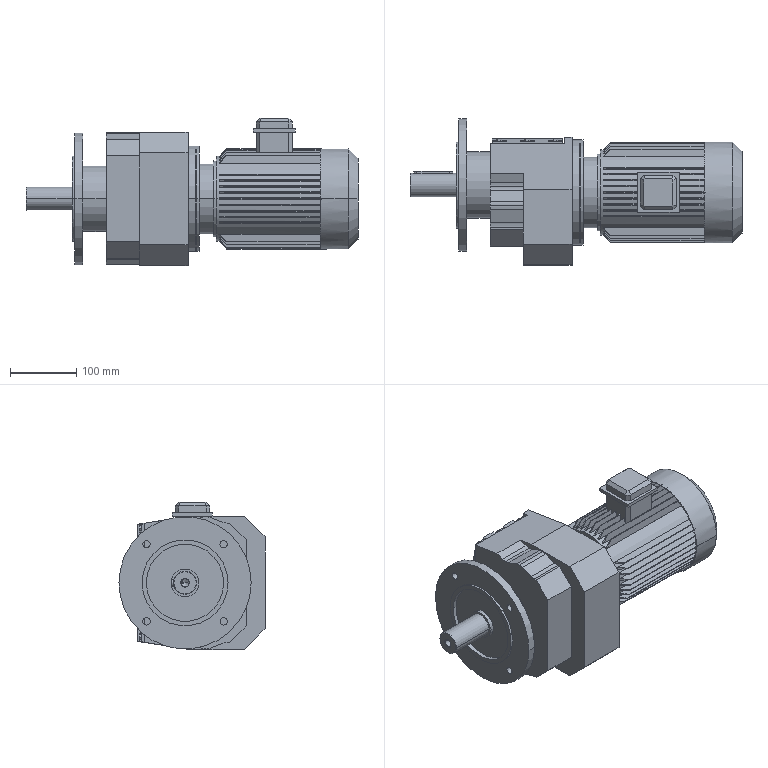Part | STEP file | NRFNRF57_NRF 27 | 1 solid | 478 faces | box 502 x 221 x 222.6 mm | volume 8380262 mm3 | plane 334 | cone 98 | cylinder 46 | commonest cylinder face diameters 11 x8 38.211 x8 160 x4 10 x2 12 x2 35 x2